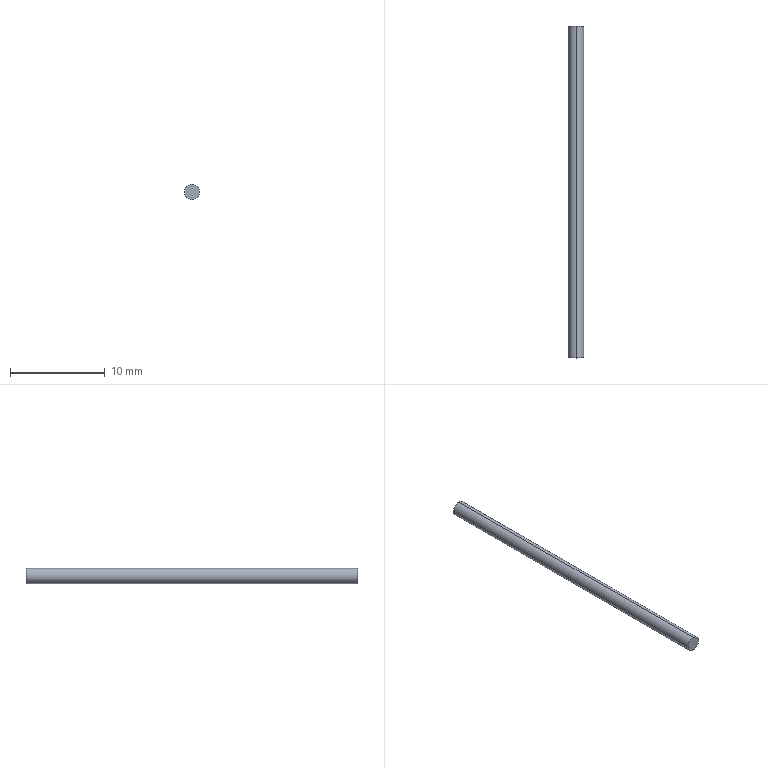Part | SolidWorks | features Extrusion 1 | 1 solid | 4 faces | box 1.6 x 35 x 1.6 mm | volume 70.372 mm3 | cylinder 2 | plane 2 | commonest cylinder face diameters 1.6 x2
STEP:
#1=CARTESIAN_POINT('',(0.,35.,0.8));
#2=VERTEX_POINT('',#1);
#3=CARTESIAN_POINT('',(0.,35.,-0.8));
#4=VERTEX_POINT('',#3);
#5=CARTESIAN_POINT('',(0.,35.,0.));
#6=DIRECTION('',(0.,1.,0.));
#7=DIRECTION('',(0.,0.,1.));
#8=AXIS2_PLACEMENT_3D('',#5,#6,#7);
#9=CIRCLE('',#8,0.8);
#10=EDGE_CURVE('',#2,#4,#9,.T.);
#11=ORIENTED_EDGE('',*,*,#10,.F.);
#12=CARTESIAN_POINT('',(0.,0.,0.8));
#13=VERTEX_POINT('',#12);
#14=CARTESIAN_POINT('',(0.,35.,0.8));
#15=DIRECTION('',(0.,-1.,0.));
#16=VECTOR('',#15,1000.);
#17=LINE('',#14,#16);
#18=EDGE_CURVE('',#2,#13,#17,.T.);
#19=ORIENTED_EDGE('',*,*,#18,.T.);
#20=CARTESIAN_POINT('',(0.,0.,-0.8));
#21=VERTEX_POINT('',#20);
#22=CARTESIAN_POINT('',(0.,0.,0.));
#23=DIRECTION('',(0.,1.,0.));
#24=DIRECTION('',(0.,0.,1.));
#25=AXIS2_PLACEMENT_3D('',#22,#23,#24);
#26=CIRCLE('',#25,0.8);
#27=EDGE_CURVE('',#13,#21,#26,.T.);
#28=ORIENTED_EDGE('',*,*,#27,.T.);
#29=CARTESIAN_POINT('',(0.,35.,-0.8));
#30=DIRECTION('',(0.,-1.,0.));
#31=VECTOR('',#30,1000.);
#32=LINE('',#29,#31);
#33=EDGE_CURVE('',#4,#21,#32,.T.);
#34=ORIENTED_EDGE('',*,*,#33,.F.);
#35=EDGE_LOOP('',(#11,#19,#28,#34));
#36=FACE_OUTER_BOUND('',#35,.T.);
#37=CARTESIAN_POINT('',(0.,35.,0.));
#38=DIRECTION('',(0.,-1.,0.));
#39=DIRECTION('',(0.,0.,-1.));
#40=AXIS2_PLACEMENT_3D('',#37,#38,#39);
#41=CYLINDRICAL_SURFACE('',#40,0.8);
#42=ADVANCED_FACE('',(#36),#41,.T.);
#43=ORIENTED_EDGE('',*,*,#18,.F.);
#44=CARTESIAN_POINT('',(0.,35.,0.));
#45=DIRECTION('',(0.,1.,0.));
#46=DIRECTION('',(0.,0.,1.));
#47=AXIS2_PLACEMENT_3D('',#44,#45,#46);
#48=CIRCLE('',#47,0.8);
#49=EDGE_CURVE('',#4,#2,#48,.T.);
#50=ORIENTED_EDGE('',*,*,#49,.F.);
#51=ORIENTED_EDGE('',*,*,#33,.T.);
#52=CARTESIAN_POINT('',(0.,0.,0.));
#53=DIRECTION('',(0.,1.,0.));
#54=DIRECTION('',(0.,0.,1.));
#55=AXIS2_PLACEMENT_3D('',#52,#53,#54);
#56=CIRCLE('',#55,0.8);
#57=EDGE_CURVE('',#21,#13,#56,.T.);
#58=ORIENTED_EDGE('',*,*,#57,.T.);
#59=EDGE_LOOP('',(#43,#50,#51,#58));
#60=FACE_OUTER_BOUND('',#59,.T.);
#61=CARTESIAN_POINT('',(0.,35.,0.));
#62=DIRECTION('',(0.,-1.,0.));
#63=DIRECTION('',(0.,0.,-1.));
#64=AXIS2_PLACEMENT_3D('',#61,#62,#63);
#65=CYLINDRICAL_SURFACE('',#64,0.8);
#66=ADVANCED_FACE('',(#60),#65,.T.);
#67=ORIENTED_EDGE('',*,*,#49,.T.);
#68=ORIENTED_EDGE('',*,*,#10,.T.);
#69=EDGE_LOOP('',(#67,#68));
#70=FACE_OUTER_BOUND('',#69,.T.);
#71=CARTESIAN_POINT('',(0.,35.,0.));
#72=DIRECTION('',(0.,1.,0.));
#73=DIRECTION('',(0.,0.,1.));
#74=AXIS2_PLACEMENT_3D('',#71,#72,#73);
#75=PLANE('',#74);
#76=ADVANCED_FACE('',(#70),#75,.T.);
#77=ORIENTED_EDGE('',*,*,#57,.F.);
#78=ORIENTED_EDGE('',*,*,#27,.F.);
#79=EDGE_LOOP('',(#77,#78));
#80=FACE_OUTER_BOUND('',#79,.T.);
#81=CARTESIAN_POINT('',(0.,0.,0.));
#82=DIRECTION('',(0.,1.,0.));
#83=DIRECTION('',(0.,0.,1.));
#84=AXIS2_PLACEMENT_3D('',#81,#82,#83);
#85=PLANE('',#84);
#86=ADVANCED_FACE('',(#80),#85,.F.);
#87=CLOSED_SHELL('',(#42,#66,#76,#86));
#88=MANIFOLD_SOLID_BREP('',#87);
#89=CARTESIAN_POINT('',(0.,0.,0.));
#90=DIRECTION('',(0.,0.,1.));
#91=DIRECTION('',(1.,0.,0.));
#92=AXIS2_PLACEMENT_3D('',#89,#90,#91);
#93=(LENGTH_UNIT()NAMED_UNIT(*)SI_UNIT(.MILLI.,.METRE.));
#94=UNCERTAINTY_MEASURE_WITH_UNIT(LENGTH_MEASURE(0.00001),#93,'','');
#95=(NAMED_UNIT(*)PLANE_ANGLE_UNIT()SI_UNIT($,.RADIAN.));
#96=(NAMED_UNIT(*)SI_UNIT($,.STERADIAN.)SOLID_ANGLE_UNIT());
#97=(GEOMETRIC_REPRESENTATION_CONTEXT(3)GLOBAL_UNCERTAINTY_ASSIGNED_CONTEXT((#94))GLOBAL_UNIT_ASSIGNED_CONTEXT((#93,#95,#96))REPRESENTATION_CONTEXT('',''));
#98=ADVANCED_BREP_SHAPE_REPRESENTATION('',(#88,#92),#97);